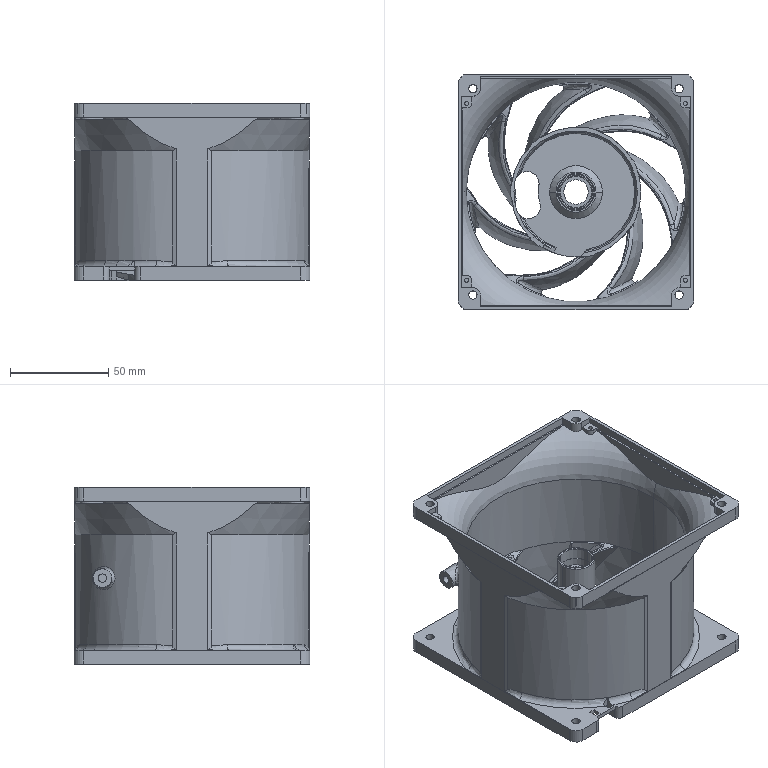NC program | NX | posted with a generic post | part box 120 x 120 x 90.2 mm
Lines 26780 to 27866 of 828686:
(等高精加工_COPY_COPY , TOOL : 10R0.5)
N53552 T07 M6
N53554 G54
N53556 G17 G0 G90 X5. Y48.5 S6800 M3
N53558 G43 Z140.7 H7
N53560 Z91.1
N53562 G94 G1 Z90.1 F3500.
N53564 X4.964 Y49.103
N53566 X4.855 Y49.697
N53568 X4.675 Y50.273
N53570 X4.427 Y50.824
N53572 X4.115 Y51.34
N53574 X3.743 Y51.816
N53576 X3.316 Y52.243
N53578 X2.84 Y52.615
N53580 X2.324 Y52.927
N53582 X1.773 Y53.175
N53584 X1.197 Y53.355
N53586 X0.603 Y53.464
N53588 X0. Y53.5
N53590 X-43.7
N53592 X-43.698 Y52.684
N53594 X-43.744 Y51.87
N53596 X-43.844 Y51.126
N53598 X-44.005 Y50.394
N53600 X-44.228 Y49.677
N53602 X-44.509 Y48.982
N53604 X-44.847 Y48.312
N53606 X-45.24 Y47.673
N53608 X-45.686 Y47.069
N53610 X-46.18 Y46.504
N53612 X-46.747 Y45.956
N53614 X-47.361 Y45.46
N53616 X-48.016 Y45.02
N53618 X-48.707 Y44.639
N53620 X-49.429 Y44.32
N53622 X-50.176 Y44.066
N53624 X-51.005 Y43.866
N53626 X-51.849 Y43.744
N53628 X-52.7 Y43.7
N53630 X-53.5
N53632 Y-43.7
N53634 X-52.715 Y-43.695
N53636 X-51.932 Y-43.74
N53638 X-51.153 Y-43.835
N53640 X-50.42 Y-43.998
N53642 X-49.704 Y-44.219
N53644 X-49.007 Y-44.497
N53646 X-48.32 Y-44.843
N53648 X-47.665 Y-45.246
N53650 X-47.047 Y-45.703
N53652 X-46.47 Y-46.212
N53654 X-45.939 Y-46.768
N53656 X-45.457 Y-47.367
N53658 X-45.028 Y-48.005
N53660 X-44.756 Y-48.481
N53662 X-44.603 Y-48.77
N53664 X-44.471 Y-49.068
N53666 X-44.357 Y-49.348
N53668 X-44.122 Y-49.997
N53670 X-43.938 Y-50.662
N53672 X-43.806 Y-51.34
N53674 X-43.727 Y-52.025
N53676 X-43.7 Y-52.715
N53678 Y-53.43
N53680 X-43.701 Y-53.501
N53682 X43.7 Y-53.5
N53684 X43.699 Y-52.682
N53686 X43.744 Y-51.865
N53688 X43.834 Y-51.176
N53690 X43.978 Y-50.496
N53692 X44.175 Y-49.83
N53694 X44.425 Y-49.182
N53696 X44.621 Y-48.736
N53698 X44.854 Y-48.308
N53700 X45.287 Y-47.605
N53702 X45.783 Y-46.946
N53704 X46.239 Y-46.442
N53706 X46.73 Y-45.973
N53708 X47.254 Y-45.54
N53710 X47.808 Y-45.147
N53712 X48.657 Y-44.66
N53714 X49.374 Y-44.341
N53716 X50.115 Y-44.084
N53718 X50.875 Y-43.892
N53720 X51.65 Y-43.766
N53722 X52.432 Y-43.706
N53724 X52.633 Y-43.701
N53726 X53.5 Y-43.7
N53728 Y43.7
N53730 X52.76 Y43.694
N53732 X52.02 Y43.732
N53734 X51.284 Y43.815
N53736 X50.466 Y43.984
N53738 X49.668 Y44.23
N53740 X48.896 Y44.549
N53742 X48.158 Y44.939
N53744 X47.522 Y45.343
N53746 X46.925 Y45.803
N53748 X46.372 Y46.313
N53750 X45.858 Y46.859
N53752 X45.395 Y47.448
N53754 X44.987 Y48.077
N53756 X44.602 Y48.784
N53758 X44.283 Y49.523
N53760 X44.033 Y50.288
N53762 X43.853 Y51.073
N53764 X43.745 Y51.87
N53766 X43.698 Y52.684
N53768 X43.7 Y53.5
N53770 X0.
N53772 Z89.95
N53774 X43.7
N53776 X43.697 Y52.909
N53778 X43.71 Y52.317
N53780 X43.784 Y51.492
N53782 X43.933 Y50.678
N53784 X44.157 Y49.88
N53786 X44.453 Y49.107
N53788 X44.819 Y48.364
N53790 X45.251 Y47.657
N53792 X45.747 Y46.993
N53794 X46.301 Y46.378
N53796 X46.909 Y45.816
N53798 X47.567 Y45.312
N53800 X48.268 Y44.871
N53802 X49.006 Y44.496
N53804 X49.699 Y44.219
N53806 X50.412 Y44.
N53808 X51.14 Y43.84
N53810 X51.879 Y43.74
N53812 X52.624 Y43.701
N53814 X52.7 Y43.7
N53816 X53.5
N53818 Y-43.7
N53820 X52.633 Y-43.701
N53822 X52.432 Y-43.706
N53824 X51.671 Y-43.763
N53826 X50.917 Y-43.883
N53828 X50.176 Y-44.065
N53830 X50.132 Y-44.078
N53832 X49.45 Y-44.308
N53834 X48.79 Y-44.596
N53836 X48.158 Y-44.94
N53838 X47.698 Y-45.218
N53840 X47.265 Y-45.537
N53842 X46.757 Y-45.948
N53844 X46.281 Y-46.396
N53846 X45.841 Y-46.879
N53848 X45.439 Y-47.393
N53850 X44.992 Y-48.064
N53852 X44.606 Y-48.773
N53854 X44.287 Y-49.514
N53856 X44.035 Y-50.28
N53858 X43.853 Y-51.066
N53860 X43.743 Y-51.865
N53862 X43.699 Y-52.682
N53864 X43.7 Y-53.5
N53866 X-43.701 Y-53.501
N53868 X-43.7 Y-53.43
N53870 Y-52.7
N53872 X-43.739 Y-51.878
N53874 X-43.853 Y-51.063
N53876 X-44.041 Y-50.261
N53878 X-44.301 Y-49.48
N53880 X-44.63 Y-48.726
N53882 X-45.027 Y-48.005
N53884 X-45.456 Y-47.367
N53886 X-45.938 Y-46.767
N53888 X-46.469 Y-46.211
N53890 X-47.046 Y-45.703
N53892 X-47.664 Y-45.245
N53894 X-48.319 Y-44.842
N53896 X-49.006 Y-44.496
N53898 X-49.663 Y-44.233
N53900 X-50.338 Y-44.021
N53902 X-51.027 Y-43.861
N53904 X-51.726 Y-43.756
N53906 X-52.432 Y-43.706
N53908 X-53.5 Y-43.7
N53910 Y43.7
N53912 X-52.7
N53914 X-52.63 Y43.701
N53916 X-51.802 Y43.748
N53918 X-50.982 Y43.87
N53920 X-50.176 Y44.066
N53922 X-49.441 Y44.315
N53924 X-48.73 Y44.627
N53926 X-48.049 Y45.
N53928 X-47.404 Y45.43
N53930 X-46.847 Y45.869
N53932 X-46.327 Y46.35
N53934 X-45.847 Y46.871
N53936 X-45.41 Y47.428
N53938 X-45.019 Y48.019
N53940 X-44.625 Y48.736
N53942 X-44.298 Y49.486
N53944 X-44.04 Y50.263
N53946 X-43.855 Y51.06
N53948 X-43.743 Y51.87
N53950 X-43.698 Y52.684
N53952 X-43.7 Y53.5
N53954 X0.
N53956 Z89.8
N53958 X-43.7
N53960 X-43.698 Y52.684
N53962 X-43.743 Y51.87
N53964 X-43.854 Y51.059
N53966 X-44.04 Y50.262
N53968 X-44.297 Y49.486
N53970 X-44.624 Y48.736
N53972 X-45.018 Y48.018
N53974 X-45.486 Y47.324
N53976 X-46.017 Y46.677
N53978 X-46.606 Y46.082
N53980 X-47.248 Y45.544
N53982 X-47.937 Y45.068
N53984 X-48.667 Y44.658
N53986 X-49.432 Y44.318
N53988 X-50.225 Y44.051
N53990 X-51.04 Y43.858
N53992 X-51.869 Y43.742
N53994 X-52.684 Y43.698
N53996 X-53.5 Y43.7
N53998 Y-43.7
N54000 X-52.432 Y-43.705
N54002 X-51.628 Y-43.767
N54004 X-50.832 Y-43.9
N54006 X-50.052 Y-44.103
N54008 X-49.292 Y-44.374
N54010 X-48.559 Y-44.711
N54012 X-47.855 Y-45.12
N54014 X-47.19 Y-45.59
N54016 X-46.57 Y-46.118
N54018 X-46. Y-46.7
N54020 X-45.484 Y-47.33
N54022 X-45.027 Y-48.004
N54024 X-44.63 Y-48.726
N54026 X-44.3 Y-49.48
N54028 X-44.041 Y-50.261
N54030 X-43.853 Y-51.063
N54032 X-43.739 Y-51.878
N54034 X-43.7 Y-52.7
N54036 Y-53.43
N54038 X-43.701 Y-53.501
N54040 X43.7 Y-53.5
N54042 X43.699 Y-52.682
N54044 X43.743 Y-51.865
N54046 X43.843 Y-51.121
N54048 X44.005 Y-50.388
N54050 X44.228 Y-49.671
N54052 X44.511 Y-48.976
N54054 X44.85 Y-48.306
N54056 X45.244 Y-47.667
N54058 X45.69 Y-47.064
N54060 X46.185 Y-46.499
N54062 X46.761 Y-45.944
N54064 X47.384 Y-45.443
N54066 X48.049 Y-44.999
N54068 X48.751 Y-44.616
N54070 X49.485 Y-44.297
N54072 X50.244 Y-44.045
N54074 X51.023 Y-43.862
N54076 X51.814 Y-43.749
N54078 X52.656 Y-43.697
N54080 X53.5 Y-43.7
N54082 Y43.7
N54084 X52.7
N54086 X51.962 Y43.732
N54088 X51.229 Y43.824
N54090 X50.507 Y43.975
N54092 X49.798 Y44.185
N54094 X49.11 Y44.451
N54096 X48.445 Y44.772
N54098 X47.808 Y45.147
N54100 X47.156 Y45.614
N54102 X46.548 Y46.136
N54104 X45.989 Y46.71
N54106 X45.482 Y47.332
N54108 X45.032 Y47.995
N54110 X44.662 Y48.66
N54112 X44.349 Y49.354
N54114 X44.096 Y50.072
N54116 X43.904 Y50.809
N54118 X43.775 Y51.559
N54120 X43.71 Y52.317
N54122 X43.694 Y52.908
N54124 X43.7 Y53.5
N54126 X0.
N54128 Z89.65
N54130 X43.7
N54132 Y52.7
N54134 X43.738 Y51.87
N54136 X43.853 Y51.046
N54138 X44.044 Y50.237
N54140 X44.308 Y49.449
N54142 X44.644 Y48.688
N54144 X45.048 Y47.962
N54146 X45.518 Y47.276
N54148 X46.049 Y46.637
N54150 X46.637 Y46.049
N54152 X47.276 Y45.518
N54154 X47.962 Y45.048
N54156 X48.688 Y44.644
N54158 X49.449 Y44.308
N54160 X50.237 Y44.044
N54162 X51.046 Y43.853
N54164 X51.87 Y43.738
N54166 X52.7 Y43.7
N54168 X53.5
N54170 Y-43.7
N54172 X52.7
N54174 X51.87 Y-43.738
N54176 X51.046 Y-43.853
N54178 X50.237 Y-44.044
N54180 X49.449 Y-44.308
N54182 X48.688 Y-44.644
N54184 X47.962 Y-45.048
N54186 X47.276 Y-45.518
N54188 X46.637 Y-46.049
N54190 X46.049 Y-46.637
N54192 X45.518 Y-47.276
N54194 X45.048 Y-47.962
N54196 X44.644 Y-48.688
N54198 X44.308 Y-49.449
N54200 X44.044 Y-50.237
N54202 X43.853 Y-51.046
N54204 X43.738 Y-51.87
N54206 X43.7 Y-52.7
N54208 Y-53.5
N54210 X-43.7
N54212 Y-52.7
N54214 X-43.738 Y-51.87
N54216 X-43.853 Y-51.046
N54218 X-44.044 Y-50.237
N54220 X-44.308 Y-49.449
N54222 X-44.644 Y-48.688
N54224 X-45.048 Y-47.962
N54226 X-45.518 Y-47.276
N54228 X-46.049 Y-46.637
N54230 X-46.637 Y-46.049
N54232 X-47.276 Y-45.518
N54234 X-47.962 Y-45.048
N54236 X-48.688 Y-44.644
N54238 X-49.449 Y-44.308
N54240 X-50.237 Y-44.044
N54242 X-51.046 Y-43.853
N54244 X-51.87 Y-43.738
N54246 X-52.7 Y-43.7
N54248 X-53.5
N54250 Y43.7
N54252 X-52.7
N54254 X-51.87 Y43.738
N54256 X-51.046 Y43.853
N54258 X-50.237 Y44.044
N54260 X-49.449 Y44.308
N54262 X-48.688 Y44.644
N54264 X-47.962 Y45.048
N54266 X-47.276 Y45.518
N54268 X-46.637 Y46.049
N54270 X-46.049 Y46.637
N54272 X-45.518 Y47.276
N54274 X-45.048 Y47.962
N54276 X-44.644 Y48.688
N54278 X-44.308 Y49.449
N54280 X-44.044 Y50.237
N54282 X-43.853 Y51.046
N54284 X-43.738 Y51.87
N54286 X-43.7 Y52.7
N54288 Y53.5
N54290 X0.
N54292 Z89.5
N54294 X-43.7
N54296 Y52.7
N54298 X-43.738 Y51.87
N54300 X-43.853 Y51.046
N54302 X-44.044 Y50.237
N54304 X-44.308 Y49.449
N54306 X-44.644 Y48.688
N54308 X-45.048 Y47.962
N54310 X-45.518 Y47.276
N54312 X-46.049 Y46.637
N54314 X-46.637 Y46.049
N54316 X-47.276 Y45.518
N54318 X-47.962 Y45.048
N54320 X-48.688 Y44.644
N54322 X-49.449 Y44.308
N54324 X-50.237 Y44.044
N54326 X-51.046 Y43.853
N54328 X-51.87 Y43.738
N54330 X-52.7 Y43.7
N54332 X-53.5
N54334 Y-43.7
N54336 X-52.7
N54338 X-51.87 Y-43.738
N54340 X-51.046 Y-43.853
N54342 X-50.237 Y-44.044
N54344 X-49.449 Y-44.308
N54346 X-48.688 Y-44.644
N54348 X-47.962 Y-45.048
N54350 X-47.276 Y-45.518
N54352 X-46.637 Y-46.049
N54354 X-46.049 Y-46.637
N54356 X-45.518 Y-47.276
N54358 X-45.048 Y-47.962
N54360 X-44.644 Y-48.688
N54362 X-44.308 Y-49.449
N54364 X-44.044 Y-50.237
N54366 X-43.853 Y-51.046
N54368 X-43.738 Y-51.87
N54370 X-43.7 Y-52.7
N54372 Y-53.5
N54374 X43.7
N54376 Y-52.7
N54378 X43.738 Y-51.87
N54380 X43.853 Y-51.046
N54382 X44.044 Y-50.237
N54384 X44.308 Y-49.449
N54386 X44.644 Y-48.688
N54388 X45.048 Y-47.962
N54390 X45.518 Y-47.276
N54392 X46.049 Y-46.637
N54394 X46.637 Y-46.049
N54396 X47.276 Y-45.518
N54398 X47.962 Y-45.048
N54400 X48.688 Y-44.644
N54402 X49.449 Y-44.308
N54404 X50.237 Y-44.044
N54406 X51.046 Y-43.853
N54408 X51.87 Y-43.738
N54410 X52.7 Y-43.7
N54412 X53.5
N54414 Y43.7
N54416 X52.7
N54418 X51.87 Y43.738
N54420 X51.046 Y43.853
N54422 X50.237 Y44.044
N54424 X49.449 Y44.308
N54426 X48.688 Y44.644
N54428 X47.962 Y45.048
N54430 X47.276 Y45.518
N54432 X46.637 Y46.049
N54434 X46.049 Y46.637
N54436 X45.518 Y47.276
N54438 X45.048 Y47.962
N54440 X44.644 Y48.688
N54442 X44.308 Y49.449
N54444 X44.044 Y50.237
N54446 X43.853 Y51.046
N54448 X43.738 Y51.87
N54450 X43.7 Y52.7
N54452 Y53.5
N54454 X0.
N54456 Z89.35
N54458 X43.7
N54460 Y52.7
N54462 X43.738 Y51.87
N54464 X43.853 Y51.046
N54466 X44.044 Y50.237
N54468 X44.308 Y49.449
N54470 X44.644 Y48.688
N54472 X45.048 Y47.962
N54474 X45.518 Y47.276
N54476 X46.049 Y46.637
N54478 X46.637 Y46.049
N54480 X47.276 Y45.518
N54482 X47.962 Y45.048
N54484 X48.688 Y44.644
N54486 X49.449 Y44.308
N54488 X50.237 Y44.044
N54490 X51.046 Y43.853
N54492 X51.87 Y43.738
N54494 X52.7 Y43.7
N54496 X53.5
N54498 Y-43.7
N54500 X52.7
N54502 X51.87 Y-43.738
N54504 X51.046 Y-43.853
N54506 X50.237 Y-44.044
N54508 X49.449 Y-44.308
N54510 X48.688 Y-44.644
N54512 X47.962 Y-45.048
N54514 X47.276 Y-45.518
N54516 X46.637 Y-46.049
N54518 X46.049 Y-46.637
N54520 X45.518 Y-47.276
N54522 X45.048 Y-47.962
N54524 X44.644 Y-48.688
N54526 X44.308 Y-49.449
N54528 X44.044 Y-50.237
N54530 X43.853 Y-51.046
N54532 X43.738 Y-51.87
N54534 X43.7 Y-52.7
N54536 Y-53.5
N54538 X-43.7
N54540 Y-52.7
N54542 X-43.738 Y-51.87
N54544 X-43.853 Y-51.046
N54546 X-44.044 Y-50.237
N54548 X-44.308 Y-49.449
N54550 X-44.644 Y-48.688
N54552 X-45.048 Y-47.962
N54554 X-45.518 Y-47.276
N54556 X-46.049 Y-46.637
N54558 X-46.637 Y-46.049
N54560 X-47.276 Y-45.518
N54562 X-47.962 Y-45.048
N54564 X-48.688 Y-44.644
N54566 X-49.449 Y-44.308
N54568 X-50.237 Y-44.044
N54570 X-51.046 Y-43.853
N54572 X-51.87 Y-43.738
N54574 X-52.7 Y-43.7
N54576 X-53.5
N54578 Y43.7
N54580 X-52.7
N54582 X-51.87 Y43.738
N54584 X-51.046 Y43.853
N54586 X-50.237 Y44.044
N54588 X-49.449 Y44.308
N54590 X-48.688 Y44.644
N54592 X-47.962 Y45.048
N54594 X-47.276 Y45.518
N54596 X-46.637 Y46.049
N54598 X-46.049 Y46.637
N54600 X-45.518 Y47.276
N54602 X-45.048 Y47.962
N54604 X-44.644 Y48.688
N54606 X-44.308 Y49.449
N54608 X-44.044 Y50.237
N54610 X-43.853 Y51.046
N54612 X-43.738 Y51.87
N54614 X-43.7 Y52.7
N54616 Y53.5
N54618 X0.
N54620 Z89.2
N54622 X-43.7
N54624 Y52.7
N54626 X-43.738 Y51.87
N54628 X-43.853 Y51.046
N54630 X-44.044 Y50.237
N54632 X-44.308 Y49.449
N54634 X-44.644 Y48.688
N54636 X-45.048 Y47.962
N54638 X-45.518 Y47.276
N54640 X-46.049 Y46.637
N54642 X-46.637 Y46.049
N54644 X-47.276 Y45.518
N54646 X-47.962 Y45.048
N54648 X-48.688 Y44.644
N54650 X-49.449 Y44.308
N54652 X-50.237 Y44.044
N54654 X-51.046 Y43.853
N54656 X-51.87 Y43.738
N54658 X-52.7 Y43.7
N54660 X-53.5
N54662 Y-43.7
N54664 X-52.7
N54666 X-51.87 Y-43.738
N54668 X-51.046 Y-43.853
N54670 X-50.237 Y-44.044
N54672 X-49.449 Y-44.308
N54674 X-48.688 Y-44.644
N54676 X-47.962 Y-45.048
N54678 X-47.276 Y-45.518
N54680 X-46.637 Y-46.049
N54682 X-46.049 Y-46.637
N54684 X-45.518 Y-47.276
N54686 X-45.048 Y-47.962
N54688 X-44.644 Y-48.688
N54690 X-44.308 Y-49.449
N54692 X-44.044 Y-50.237
N54694 X-43.853 Y-51.046
N54696 X-43.738 Y-51.87
N54698 X-43.7 Y-52.7
N54700 Y-53.5
N54702 X43.7
N54704 Y-52.7
N54706 X43.738 Y-51.87
N54708 X43.853 Y-51.046
N54710 X44.044 Y-50.237
N54712 X44.308 Y-49.449
N54714 X44.644 Y-48.688
N54716 X45.048 Y-47.962
N54718 X45.518 Y-47.276
N54720 X46.049 Y-46.637
N54722 X46.637 Y-46.049
N54724 X47.276 Y-45.518
N54726 X47.962 Y-45.048
N54728 X48.688 Y-44.644
N54730 X49.449 Y-44.308
N54732 X50.237 Y-44.044
N54734 X51.046 Y-43.853
N54736 X51.87 Y-43.738
N54738 X52.7 Y-43.7
N54740 X53.5
N54742 Y43.7
N54744 X52.7
N54746 X51.87 Y43.738
N54748 X51.046 Y43.853
N54750 X50.237 Y44.044
N54752 X49.449 Y44.308
N54754 X48.688 Y44.644
N54756 X47.962 Y45.048
N54758 X47.276 Y45.518
N54760 X46.637 Y46.049
N54762 X46.049 Y46.637
N54764 X45.518 Y47.276
N54766 X45.048 Y47.962
N54768 X44.644 Y48.688
N54770 X44.308 Y49.449
N54772 X44.044 Y50.237
N54774 X43.853 Y51.046
N54776 X43.738 Y51.87
N54778 X43.7 Y52.7
N54780 Y53.5
N54782 X0.
N54784 Z89.05
N54786 X43.7
N54788 Y52.7
N54790 X43.738 Y51.87
N54792 X43.853 Y51.046
N54794 X44.044 Y50.237
N54796 X44.308 Y49.449
N54798 X44.644 Y48.688
N54800 X45.048 Y47.962
N54802 X45.518 Y47.276
N54804 X46.049 Y46.637
N54806 X46.637 Y46.049
N54808 X47.276 Y45.518
N54810 X47.962 Y45.048
N54812 X48.688 Y44.644
N54814 X49.449 Y44.308
N54816 X50.237 Y44.044
N54818 X51.046 Y43.853
N54820 X51.87 Y43.738
N54822 X52.7 Y43.7
N54824 X53.5
N54826 Y-43.7
N54828 X52.7
N54830 X51.87 Y-43.738
N54832 X51.046 Y-43.853
N54834 X50.237 Y-44.044
N54836 X49.449 Y-44.308
N54838 X48.688 Y-44.644
N54840 X47.962 Y-45.048
N54842 X47.276 Y-45.518
N54844 X46.637 Y-46.049
N54846 X46.049 Y-46.637
N54848 X45.518 Y-47.276
N54850 X45.048 Y-47.962
N54852 X44.644 Y-48.688
N54854 X44.308 Y-49.449
N54856 X44.044 Y-50.237
N54858 X43.853 Y-51.046
N54860 X43.738 Y-51.87
N54862 X43.7 Y-52.7
N54864 Y-53.5
N54866 X-43.7
N54868 Y-52.7
N54870 X-43.738 Y-51.87
N54872 X-43.853 Y-51.046
N54874 X-44.044 Y-50.237
N54876 X-44.308 Y-49.449
N54878 X-44.644 Y-48.688
N54880 X-45.048 Y-47.962
N54882 X-45.518 Y-47.276
N54884 X-46.049 Y-46.637
N54886 X-46.637 Y-46.049
N54888 X-47.276 Y-45.518
N54890 X-47.962 Y-45.048
N54892 X-48.688 Y-44.644
N54894 X-49.449 Y-44.308
N54896 X-50.237 Y-44.044
N54898 X-51.046 Y-43.853
N54900 X-51.87 Y-43.738
N54902 X-52.7 Y-43.7
N54904 X-53.5
N54906 Y43.7
N54908 X-52.7
N54910 X-51.87 Y43.738
N54912 X-51.046 Y43.853
N54914 X-50.237 Y44.044
N54916 X-49.449 Y44.308
N54918 X-48.688 Y44.644
N54920 X-47.962 Y45.048
N54922 X-47.276 Y45.518
N54924 X-46.637 Y46.049
N54926 X-46.049 Y46.637
N54928 X-45.518 Y47.276
N54930 X-45.048 Y47.962
N54932 X-44.644 Y48.688
N54934 X-44.308 Y49.449
N54936 X-44.044 Y50.237
N54938 X-43.853 Y51.046
N54940 X-43.738 Y51.87
N54942 X-43.7 Y52.7
N54944 Y53.5
N54946 X0.
N54948 Z88.9
N54950 X-43.7
N54952 Y52.7
N54954 X-43.738 Y51.87
N54956 X-43.853 Y51.046
N54958 X-44.044 Y50.237
N54960 X-44.308 Y49.449
N54962 X-44.644 Y48.688
N54964 X-45.048 Y47.962
N54966 X-45.518 Y47.276
N54968 X-46.049 Y46.637
N54970 X-46.637 Y46.049
N54972 X-47.276 Y45.518
N54974 X-47.962 Y45.048
N54976 X-48.688 Y44.644
N54978 X-49.449 Y44.308
N54980 X-50.237 Y44.044
N54982 X-51.046 Y43.853
N54984 X-51.87 Y43.738
N54986 X-52.7 Y43.7
N54988 X-53.5
N54990 Y-43.7
N54992 X-52.7
N54994 X-51.87 Y-43.738
N54996 X-51.046 Y-43.853
N54998 X-50.237 Y-44.044
N55000 X-49.449 Y-44.308
N55002 X-48.688 Y-44.644
N55004 X-47.962 Y-45.048
N55006 X-47.276 Y-45.518
N55008 X-46.637 Y-46.049
N55010 X-46.049 Y-46.637
N55012 X-45.518 Y-47.276
N55014 X-45.048 Y-47.962
N55016 X-44.644 Y-48.688
N55018 X-44.308 Y-49.449
N55020 X-44.044 Y-50.237
N55022 X-43.853 Y-51.046
N55024 X-43.738 Y-51.87
N55026 X-43.7 Y-52.7
N55028 Y-53.5
N55030 X43.7
N55032 Y-52.7
N55034 X43.738 Y-51.87
N55036 X43.853 Y-51.046
N55038 X44.044 Y-50.237
N55040 X44.308 Y-49.449
N55042 X44.644 Y-48.688
N55044 X45.048 Y-47.962
N55046 X45.518 Y-47.276
N55048 X46.049 Y-46.637
N55050 X46.637 Y-46.049
N55052 X47.276 Y-45.518
N55054 X47.962 Y-45.048
N55056 X48.688 Y-44.644
N55058 X49.449 Y-44.308
N55060 X50.237 Y-44.044
N55062 X51.046 Y-43.853
N55064 X51.87 Y-43.738
N55066 X52.7 Y-43.7
N55068 X53.5
N55070 Y43.7
N55072 X52.7
N55074 X51.87 Y43.738
N55076 X51.046 Y43.853
N55078 X50.237 Y44.044
N55080 X49.449 Y44.308
N55082 X48.688 Y44.644
N55084 X47.962 Y45.048
N55086 X47.276 Y45.518
N55088 X46.637 Y46.049
N55090 X46.049 Y46.637
N55092 X45.518 Y47.276
N55094 X45.048 Y47.962
N55096 X44.644 Y48.688
N55098 X44.308 Y49.449
N55100 X44.044 Y50.237
N55102 X43.853 Y51.046
N55104 X43.738 Y51.87
N55106 X43.7 Y52.7
N55108 Y53.5
N55110 X0.
N55112 Z88.75
N55114 X43.7
N55116 Y52.7
N55118 X43.738 Y51.87
N55120 X43.853 Y51.046
N55122 X44.044 Y50.237
N55124 X44.308 Y49.449
N55126 X44.644 Y48.688
N55128 X45.048 Y47.962
N55130 X45.518 Y47.276
N55132 X46.049 Y46.637
N55134 X46.637 Y46.049
N55136 X47.276 Y45.518
N55138 X47.962 Y45.048
N55140 X48.688 Y44.644
N55142 X49.449 Y44.308
N55144 X50.237 Y44.044
N55146 X51.046 Y43.853
N55148 X51.87 Y43.738
N55150 X52.7 Y43.7
N55152 X53.5
N55154 Y-43.7
N55156 X52.7
N55158 X51.87 Y-43.738
N55160 X51.046 Y-43.853
N55162 X50.237 Y-44.044
N55164 X49.449 Y-44.308
N55166 X48.688 Y-44.644
N55168 X47.962 Y-45.048
N55170 X47.276 Y-45.518
N55172 X46.637 Y-46.049
N55174 X46.049 Y-46.637
N55176 X45.518 Y-47.276
N55178 X45.048 Y-47.962
N55180 X44.644 Y-48.688
N55182 X44.308 Y-49.449
N55184 X44.044 Y-50.237
N55186 X43.853 Y-51.046
N55188 X43.738 Y-51.87
N55190 X43.7 Y-52.7
N55192 Y-53.5
N55194 X-43.7
N55196 Y-52.7
N55198 X-43.738 Y-51.87
N55200 X-43.853 Y-51.046
N55202 X-44.044 Y-50.237
N55204 X-44.308 Y-49.449
N55206 X-44.644 Y-48.688
N55208 X-45.048 Y-47.962
N55210 X-45.518 Y-47.276
N55212 X-46.049 Y-46.637
N55214 X-46.637 Y-46.049
N55216 X-47.276 Y-45.518
N55218 X-47.962 Y-45.048
N55220 X-48.688 Y-44.644
N55222 X-49.449 Y-44.308
N55224 X-50.237 Y-44.044
N55226 X-51.046 Y-43.853
N55228 X-51.87 Y-43.738
N55230 X-52.7 Y-43.7
N55232 X-53.5
N55234 Y43.7
N55236 X-52.7
N55238 X-51.87 Y43.738
N55240 X-51.046 Y43.853
N55242 X-50.237 Y44.044
N55244 X-49.449 Y44.308
N55246 X-48.688 Y44.644
N55248 X-47.962 Y45.048
N55250 X-47.276 Y45.518
N55252 X-46.637 Y46.049
N55254 X-46.049 Y46.637
N55256 X-45.518 Y47.276
N55258 X-45.048 Y47.962
N55260 X-44.644 Y48.688
N55262 X-44.308 Y49.449
N55264 X-44.044 Y50.237
N55266 X-43.853 Y51.046
N55268 X-43.738 Y51.87
N55270 X-43.7 Y52.7
N55272 Y53.5
N55274 X0.
N55276 Z88.6
N55278 X-43.7
N55280 Y52.7
N55282 X-43.738 Y51.87
N55284 X-43.853 Y51.046
N55286 X-44.044 Y50.237
N55288 X-44.308 Y49.449
N55290 X-44.644 Y48.688
N55292 X-45.048 Y47.962
N55294 X-45.518 Y47.276
N55296 X-46.049 Y46.637
N55298 X-46.637 Y46.049
N55300 X-47.276 Y45.518
N55302 X-47.962 Y45.048
N55304 X-48.688 Y44.644
N55306 X-49.449 Y44.308
N55308 X-50.237 Y44.044
N55310 X-51.046 Y43.853
N55312 X-51.87 Y43.738
N55314 X-52.7 Y43.7
N55316 X-53.5
N55318 Y-43.7
N55320 X-52.7
N55322 X-51.87 Y-43.738
N55324 X-51.046 Y-43.853
N55326 X-50.237 Y-44.044
N55328 X-49.449 Y-44.308
N55330 X-48.688 Y-44.644
N55332 X-47.962 Y-45.048
N55334 X-47.276 Y-45.518
N55336 X-46.637 Y-46.049
N55338 X-46.049 Y-46.637
N55340 X-45.518 Y-47.276
N55342 X-45.048 Y-47.962
N55344 X-44.644 Y-48.688
N55346 X-44.308 Y-49.449
N55348 X-44.044 Y-50.237
N55350 X-43.853 Y-51.046
N55352 X-43.738 Y-51.87
N55354 X-43.7 Y-52.7
N55356 Y-53.5
N55358 X43.7
N55360 Y-52.7
N55362 X43.738 Y-51.87
N55364 X43.853 Y-51.046
N55366 X44.044 Y-50.237
N55368 X44.308 Y-49.449
N55370 X44.644 Y-48.688
N55372 X45.048 Y-47.962
N55374 X45.518 Y-47.276
N55376 X46.049 Y-46.637
N55378 X46.637 Y-46.049
N55380 X47.276 Y-45.518
N55382 X47.962 Y-45.048
N55384 X48.688 Y-44.644
N55386 X49.449 Y-44.308
N55388 X50.237 Y-44.044
N55390 X51.046 Y-43.853
N55392 X51.87 Y-43.738
N55394 X52.7 Y-43.7
N55396 X53.5
N55398 Y43.7
N55400 X52.7
N55402 X51.87 Y43.738
N55404 X51.046 Y43.853
N55406 X50.237 Y44.044
N55408 X49.449 Y44.308
N55410 X48.688 Y44.644
N55412 X47.962 Y45.048
N55414 X47.276 Y45.518
N55416 X46.637 Y46.049
N55418 X46.049 Y46.637
N55420 X45.518 Y47.276
N55422 X45.048 Y47.962
N55424 X44.644 Y48.688
N55426 X44.308 Y49.449
N55428 X44.044 Y50.237
N55430 X43.853 Y51.046
N55432 X43.738 Y51.87
N55434 X43.7 Y52.7
N55436 Y53.5
N55438 X0.
N55440 Z88.45
N55442 X43.7
N55444 Y52.7
N55446 X43.738 Y51.87
N55448 X43.853 Y51.046
N55450 X44.044 Y50.237
N55452 X44.308 Y49.449
N55454 X44.644 Y48.688
N55456 X45.048 Y47.962
N55458 X45.518 Y47.276
N55460 X46.049 Y46.637
N55462 X46.637 Y46.049
N55464 X47.276 Y45.518
N55466 X47.962 Y45.048
N55468 X48.688 Y44.644
N55470 X49.449 Y44.308
N55472 X50.237 Y44.044
N55474 X51.046 Y43.853
N55476 X51.87 Y43.738
N55478 X52.7 Y43.7
N55480 X53.5
N55482 Y-43.7
N55484 X52.7
N55486 X51.87 Y-43.738
N55488 X51.046 Y-43.853
N55490 X50.237 Y-44.044
N55492 X49.449 Y-44.308
N55494 X48.688 Y-44.644
N55496 X47.962 Y-45.048
N55498 X47.276 Y-45.518
N55500 X46.637 Y-46.049
N55502 X46.049 Y-46.637
N55504 X45.518 Y-47.276
N55506 X45.048 Y-47.962
N55508 X44.644 Y-48.688
N55510 X44.308 Y-49.449
N55512 X44.044 Y-50.237
N55514 X43.853 Y-51.046
N55516 X43.738 Y-51.87
N55518 X43.7 Y-52.7
N55520 Y-53.5
N55522 X-43.7
N55524 Y-52.7
N55526 X-43.738 Y-51.87
N55528 X-43.853 Y-51.046
N55530 X-44.044 Y-50.237
N55532 X-44.308 Y-49.449
N55534 X-44.644 Y-48.688
N55536 X-45.048 Y-47.962
N55538 X-45.518 Y-47.276
N55540 X-46.049 Y-46.637
N55542 X-46.637 Y-46.049
N55544 X-47.276 Y-45.518
N55546 X-47.962 Y-45.048
N55548 X-48.688 Y-44.644
N55550 X-49.449 Y-44.308
N55552 X-50.237 Y-44.044
N55554 X-51.046 Y-43.853
N55556 X-51.87 Y-43.738
N55558 X-52.7 Y-43.7
N55560 X-53.5
N55562 Y43.7
N55564 X-52.7
N55566 X-51.87 Y43.738
N55568 X-51.046 Y43.853
N55570 X-50.237 Y44.044
N55572 X-49.449 Y44.308
N55574 X-48.688 Y44.644
N55576 X-47.962 Y45.048
N55578 X-47.276 Y45.518
N55580 X-46.637 Y46.049
N55582 X-46.049 Y46.637
N55584 X-45.518 Y47.276
N55586 X-45.048 Y47.962
N55588 X-44.644 Y48.688
N55590 X-44.308 Y49.449
N55592 X-44.044 Y50.237
N55594 X-43.853 Y51.046
N55596 X-43.738 Y51.87
N55598 X-43.7 Y52.7
N55600 Y53.5
N55602 X0.
N55604 Z88.3
N55606 X-43.7
N55608 Y52.7
N55610 X-43.738 Y51.87
N55612 X-43.853 Y51.046
N55614 X-44.044 Y50.237
N55616 X-44.308 Y49.449
N55618 X-44.644 Y48.688
N55620 X-45.048 Y47.962
N55622 X-45.518 Y47.276
N55624 X-46.049 Y46.637
N55626 X-46.637 Y46.049
N55628 X-47.276 Y45.518
N55630 X-47.962 Y45.048
N55632 X-48.688 Y44.644
N55634 X-49.449 Y44.308
N55636 X-50.237 Y44.044
N55638 X-51.046 Y43.853
N55640 X-51.87 Y43.738
N55642 X-52.7 Y43.7
N55644 X-53.5
N55646 Y-43.7
N55648 X-52.7
N55650 X-51.87 Y-43.738
N55652 X-51.046 Y-43.853
N55654 X-50.237 Y-44.044
N55656 X-49.449 Y-44.308
N55658 X-48.688 Y-44.644
N55660 X-47.962 Y-45.048
N55662 X-47.276 Y-45.518
N55664 X-46.637 Y-46.049
N55666 X-46.049 Y-46.637
N55668 X-45.518 Y-47.276
N55670 X-45.048 Y-47.962
N55672 X-44.644 Y-48.688
N55674 X-44.308 Y-49.449
N55676 X-44.044 Y-50.237
N55678 X-43.853 Y-51.046
N55680 X-43.738 Y-51.87
N55682 X-43.7 Y-52.7
N55684 Y-53.5
N55686 X43.7
N55688 Y-52.7
N55690 X43.738 Y-51.87
N55692 X43.853 Y-51.046
N55694 X44.044 Y-50.237
N55696 X44.308 Y-49.449
N55698 X44.644 Y-48.688
N55700 X45.048 Y-47.962
N55702 X45.518 Y-47.276
N55704 X46.049 Y-46.637
N55706 X46.637 Y-46.049
N55708 X47.276 Y-45.518
N55710 X47.962 Y-45.048
N55712 X48.688 Y-44.644
N55714 X49.449 Y-44.308
N55716 X50.237 Y-44.044
N55718 X51.046 Y-43.853